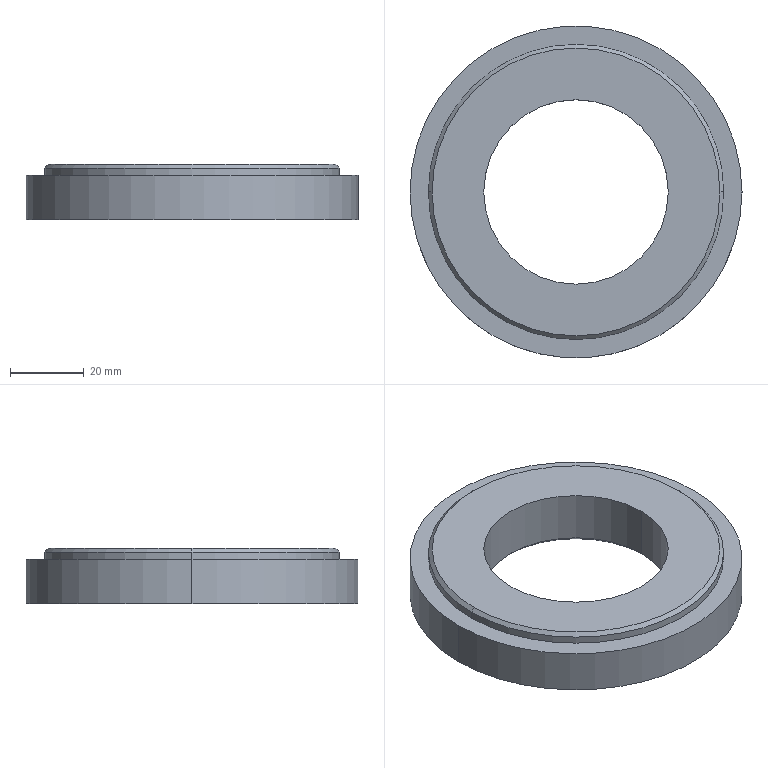Part | SolidWorks | features ICE 2, Chamfer 1, Extrusion 1 | 1 solid | 31 faces | box 90 x 90 x 15 mm | volume 60934 mm3 | cylinder 18 | plane 9 | cone 4 | commonest cylinder face diameters 4 x12 50 x2 80 x2 90 x2
STEP:
#1=CARTESIAN_POINT('',(39.,0.,15.));
#2=VERTEX_POINT('',#1);
#3=CARTESIAN_POINT('',(-39.,0.,15.));
#4=VERTEX_POINT('',#3);
#5=CARTESIAN_POINT('',(0.,0.,15.));
#6=DIRECTION('',(0.,0.,1.));
#7=DIRECTION('',(1.,0.,0.));
#8=AXIS2_PLACEMENT_3D('',#5,#6,#7);
#9=CIRCLE('',#8,39.);
#10=EDGE_CURVE('',#2,#4,#9,.T.);
#11=ORIENTED_EDGE('',*,*,#10,.F.);
#12=CARTESIAN_POINT('',(40.,0.,14.));
#13=VERTEX_POINT('',#12);
#14=CARTESIAN_POINT('',(39.,0.,15.));
#15=DIRECTION('',(0.7071,0.,-0.7071));
#16=VECTOR('',#15,1000.);
#17=LINE('',#14,#16);
#18=EDGE_CURVE('',#2,#13,#17,.T.);
#19=ORIENTED_EDGE('',*,*,#18,.T.);
#20=CARTESIAN_POINT('',(-40.,0.,14.));
#21=VERTEX_POINT('',#20);
#22=CARTESIAN_POINT('',(0.,0.,14.));
#23=DIRECTION('',(0.,0.,-1.));
#24=DIRECTION('',(1.,0.,0.));
#25=AXIS2_PLACEMENT_3D('',#22,#23,#24);
#26=CIRCLE('',#25,40.);
#27=EDGE_CURVE('',#21,#13,#26,.T.);
#28=ORIENTED_EDGE('',*,*,#27,.F.);
#29=CARTESIAN_POINT('',(-39.,0.,15.));
#30=DIRECTION('',(-0.7071,0.,-0.7071));
#31=VECTOR('',#30,1000.);
#32=LINE('',#29,#31);
#33=EDGE_CURVE('',#4,#21,#32,.T.);
#34=ORIENTED_EDGE('',*,*,#33,.F.);
#35=EDGE_LOOP('',(#11,#19,#28,#34));
#36=FACE_OUTER_BOUND('',#35,.T.);
#37=CARTESIAN_POINT('',(0.,0.,15.));
#38=DIRECTION('',(0.,0.,-1.));
#39=DIRECTION('',(-1.,0.,0.));
#40=AXIS2_PLACEMENT_3D('',#37,#38,#39);
#41=CONICAL_SURFACE('',#40,39.,0.7854);
#42=ADVANCED_FACE('',(#36),#41,.T.);
#43=CARTESIAN_POINT('',(25.,0.,1.));
#44=VERTEX_POINT('',#43);
#45=CARTESIAN_POINT('',(-25.,0.,1.));
#46=VERTEX_POINT('',#45);
#47=CARTESIAN_POINT('',(0.,0.,1.));
#48=DIRECTION('',(0.,0.,-1.));
#49=DIRECTION('',(1.,0.,0.));
#50=AXIS2_PLACEMENT_3D('',#47,#48,#49);
#51=CIRCLE('',#50,25.);
#52=EDGE_CURVE('',#44,#46,#51,.T.);
#53=ORIENTED_EDGE('',*,*,#52,.F.);
#54=CARTESIAN_POINT('',(26.,0.,0.));
#55=VERTEX_POINT('',#54);
#56=CARTESIAN_POINT('',(26.,0.,0.));
#57=DIRECTION('',(0.7071,0.,-0.7071));
#58=VECTOR('',#57,1000.);
#59=LINE('',#56,#58);
#60=EDGE_CURVE('',#44,#55,#59,.T.);
#61=ORIENTED_EDGE('',*,*,#60,.T.);
#62=CARTESIAN_POINT('',(-26.,0.,0.));
#63=VERTEX_POINT('',#62);
#64=CARTESIAN_POINT('',(0.,0.,0.));
#65=DIRECTION('',(0.,0.,1.));
#66=DIRECTION('',(1.,0.,0.));
#67=AXIS2_PLACEMENT_3D('',#64,#65,#66);
#68=CIRCLE('',#67,26.);
#69=EDGE_CURVE('',#63,#55,#68,.T.);
#70=ORIENTED_EDGE('',*,*,#69,.F.);
#71=CARTESIAN_POINT('',(-26.,0.,0.));
#72=DIRECTION('',(-0.7071,0.,-0.7071));
#73=VECTOR('',#72,1000.);
#74=LINE('',#71,#73);
#75=EDGE_CURVE('',#46,#63,#74,.T.);
#76=ORIENTED_EDGE('',*,*,#75,.F.);
#77=EDGE_LOOP('',(#53,#61,#70,#76));
#78=FACE_OUTER_BOUND('',#77,.T.);
#79=CARTESIAN_POINT('',(0.,0.,0.));
#80=DIRECTION('',(0.,0.,-1.));
#81=DIRECTION('',(-1.,0.,0.));
#82=AXIS2_PLACEMENT_3D('',#79,#80,#81);
#83=CONICAL_SURFACE('',#82,26.,0.7854);
#84=ADVANCED_FACE('',(#78),#83,.F.);
#85=CARTESIAN_POINT('',(33.61,18.25,11.));
#86=VERTEX_POINT('',#85);
#87=CARTESIAN_POINT('',(29.61,18.25,11.));
#88=VERTEX_POINT('',#87);
#89=CARTESIAN_POINT('',(31.61,18.25,11.));
#90=DIRECTION('',(0.,0.,-1.));
#91=DIRECTION('',(-1.,0.,0.));
#92=AXIS2_PLACEMENT_3D('',#89,#90,#91);
#93=CIRCLE('',#92,2.);
#94=EDGE_CURVE('',#86,#88,#93,.T.);
#95=ORIENTED_EDGE('',*,*,#94,.F.);
#96=CARTESIAN_POINT('',(33.61,18.25,0.));
#97=VERTEX_POINT('',#96);
#98=CARTESIAN_POINT('',(33.61,18.25,11.));
#99=DIRECTION('',(0.,0.,-1.));
#100=VECTOR('',#99,1000.);
#101=LINE('',#98,#100);
#102=EDGE_CURVE('',#86,#97,#101,.T.);
#103=ORIENTED_EDGE('',*,*,#102,.T.);
#104=CARTESIAN_POINT('',(29.61,18.25,0.));
#105=VERTEX_POINT('',#104);
#106=CARTESIAN_POINT('',(31.61,18.25,0.));
#107=DIRECTION('',(0.,0.,-1.));
#108=DIRECTION('',(-1.,0.,0.));
#109=AXIS2_PLACEMENT_3D('',#106,#107,#108);
#110=CIRCLE('',#109,2.);
#111=EDGE_CURVE('',#97,#105,#110,.T.);
#112=ORIENTED_EDGE('',*,*,#111,.T.);
#113=CARTESIAN_POINT('',(29.61,18.25,11.));
#114=DIRECTION('',(0.,0.,-1.));
#115=VECTOR('',#114,1000.);
#116=LINE('',#113,#115);
#117=EDGE_CURVE('',#88,#105,#116,.T.);
#118=ORIENTED_EDGE('',*,*,#117,.F.);
#119=EDGE_LOOP('',(#95,#103,#112,#118));
#120=FACE_OUTER_BOUND('',#119,.T.);
#121=CARTESIAN_POINT('',(31.61,18.25,11.));
#122=DIRECTION('',(0.,0.,-1.));
#123=DIRECTION('',(-1.,0.,0.));
#124=AXIS2_PLACEMENT_3D('',#121,#122,#123);
#125=CYLINDRICAL_SURFACE('',#124,2.);
#126=ADVANCED_FACE('',(#120),#125,.F.);
#127=CARTESIAN_POINT('',(33.61,-18.25,11.));
#128=VERTEX_POINT('',#127);
#129=CARTESIAN_POINT('',(29.61,-18.25,11.));
#130=VERTEX_POINT('',#129);
#131=CARTESIAN_POINT('',(31.61,-18.25,11.));
#132=DIRECTION('',(0.,0.,-1.));
#133=DIRECTION('',(-1.,0.,0.));
#134=AXIS2_PLACEMENT_3D('',#131,#132,#133);
#135=CIRCLE('',#134,2.);
#136=EDGE_CURVE('',#128,#130,#135,.T.);
#137=ORIENTED_EDGE('',*,*,#136,.F.);
#138=CARTESIAN_POINT('',(33.61,-18.25,0.));
#139=VERTEX_POINT('',#138);
#140=CARTESIAN_POINT('',(33.61,-18.25,11.));
#141=DIRECTION('',(0.,0.,-1.));
#142=VECTOR('',#141,1000.);
#143=LINE('',#140,#142);
#144=EDGE_CURVE('',#128,#139,#143,.T.);
#145=ORIENTED_EDGE('',*,*,#144,.T.);
#146=CARTESIAN_POINT('',(29.61,-18.25,0.));
#147=VERTEX_POINT('',#146);
#148=CARTESIAN_POINT('',(31.61,-18.25,0.));
#149=DIRECTION('',(0.,0.,-1.));
#150=DIRECTION('',(-1.,0.,0.));
#151=AXIS2_PLACEMENT_3D('',#148,#149,#150);
#152=CIRCLE('',#151,2.);
#153=EDGE_CURVE('',#139,#147,#152,.T.);
#154=ORIENTED_EDGE('',*,*,#153,.T.);
#155=CARTESIAN_POINT('',(29.61,-18.25,11.));
#156=DIRECTION('',(0.,0.,-1.));
#157=VECTOR('',#156,1000.);
#158=LINE('',#155,#157);
#159=EDGE_CURVE('',#130,#147,#158,.T.);
#160=ORIENTED_EDGE('',*,*,#159,.F.);
#161=EDGE_LOOP('',(#137,#145,#154,#160));
#162=FACE_OUTER_BOUND('',#161,.T.);
#163=CARTESIAN_POINT('',(31.61,-18.25,11.));
#164=DIRECTION('',(0.,0.,-1.));
#165=DIRECTION('',(-1.,0.,0.));
#166=AXIS2_PLACEMENT_3D('',#163,#164,#165);
#167=CYLINDRICAL_SURFACE('',#166,2.);
#168=ADVANCED_FACE('',(#162),#167,.F.);
#169=CARTESIAN_POINT('',(2.,-36.5,11.));
#170=VERTEX_POINT('',#169);
#171=CARTESIAN_POINT('',(-2.,-36.5,11.));
#172=VERTEX_POINT('',#171);
#173=CARTESIAN_POINT('',(0.,-36.5,11.));
#174=DIRECTION('',(0.,0.,-1.));
#175=DIRECTION('',(-1.,0.,0.));
#176=AXIS2_PLACEMENT_3D('',#173,#174,#175);
#177=CIRCLE('',#176,2.);
#178=EDGE_CURVE('',#170,#172,#177,.T.);
#179=ORIENTED_EDGE('',*,*,#178,.F.);
#180=CARTESIAN_POINT('',(2.,-36.5,0.));
#181=VERTEX_POINT('',#180);
#182=CARTESIAN_POINT('',(2.,-36.5,11.));
#183=DIRECTION('',(0.,0.,-1.));
#184=VECTOR('',#183,1000.);
#185=LINE('',#182,#184);
#186=EDGE_CURVE('',#170,#181,#185,.T.);
#187=ORIENTED_EDGE('',*,*,#186,.T.);
#188=CARTESIAN_POINT('',(-2.,-36.5,0.));
#189=VERTEX_POINT('',#188);
#190=CARTESIAN_POINT('',(0.,-36.5,0.));
#191=DIRECTION('',(0.,0.,-1.));
#192=DIRECTION('',(-1.,0.,0.));
#193=AXIS2_PLACEMENT_3D('',#190,#191,#192);
#194=CIRCLE('',#193,2.);
#195=EDGE_CURVE('',#181,#189,#194,.T.);
#196=ORIENTED_EDGE('',*,*,#195,.T.);
#197=CARTESIAN_POINT('',(-2.,-36.5,11.));
#198=DIRECTION('',(0.,0.,-1.));
#199=VECTOR('',#198,1000.);
#200=LINE('',#197,#199);
#201=EDGE_CURVE('',#172,#189,#200,.T.);
#202=ORIENTED_EDGE('',*,*,#201,.F.);
#203=EDGE_LOOP('',(#179,#187,#196,#202));
#204=FACE_OUTER_BOUND('',#203,.T.);
#205=CARTESIAN_POINT('',(0.,-36.5,11.));
#206=DIRECTION('',(0.,0.,-1.));
#207=DIRECTION('',(-1.,0.,0.));
#208=AXIS2_PLACEMENT_3D('',#205,#206,#207);
#209=CYLINDRICAL_SURFACE('',#208,2.);
#210=ADVANCED_FACE('',(#204),#209,.F.);
#211=CARTESIAN_POINT('',(-29.61,-18.25,11.));
#212=VERTEX_POINT('',#211);
#213=CARTESIAN_POINT('',(-33.61,-18.25,11.));
#214=VERTEX_POINT('',#213);
#215=CARTESIAN_POINT('',(-31.61,-18.25,11.));
#216=DIRECTION('',(0.,0.,-1.));
#217=DIRECTION('',(-1.,0.,0.));
#218=AXIS2_PLACEMENT_3D('',#215,#216,#217);
#219=CIRCLE('',#218,2.);
#220=EDGE_CURVE('',#212,#214,#219,.T.);
#221=ORIENTED_EDGE('',*,*,#220,.F.);
#222=CARTESIAN_POINT('',(-29.61,-18.25,0.));
#223=VERTEX_POINT('',#222);
#224=CARTESIAN_POINT('',(-29.61,-18.25,11.));
#225=DIRECTION('',(0.,0.,-1.));
#226=VECTOR('',#225,1000.);
#227=LINE('',#224,#226);
#228=EDGE_CURVE('',#212,#223,#227,.T.);
#229=ORIENTED_EDGE('',*,*,#228,.T.);
#230=CARTESIAN_POINT('',(-33.61,-18.25,0.));
#231=VERTEX_POINT('',#230);
#232=CARTESIAN_POINT('',(-31.61,-18.25,0.));
#233=DIRECTION('',(0.,0.,-1.));
#234=DIRECTION('',(-1.,0.,0.));
#235=AXIS2_PLACEMENT_3D('',#232,#233,#234);
#236=CIRCLE('',#235,2.);
#237=EDGE_CURVE('',#223,#231,#236,.T.);
#238=ORIENTED_EDGE('',*,*,#237,.T.);
#239=CARTESIAN_POINT('',(-33.61,-18.25,11.));
#240=DIRECTION('',(0.,0.,-1.));
#241=VECTOR('',#240,1000.);
#242=LINE('',#239,#241);
#243=EDGE_CURVE('',#214,#231,#242,.T.);
#244=ORIENTED_EDGE('',*,*,#243,.F.);
#245=EDGE_LOOP('',(#221,#229,#238,#244));
#246=FACE_OUTER_BOUND('',#245,.T.);
#247=CARTESIAN_POINT('',(-31.61,-18.25,11.));
#248=DIRECTION('',(0.,0.,-1.));
#249=DIRECTION('',(-1.,0.,0.));
#250=AXIS2_PLACEMENT_3D('',#247,#248,#249);
#251=CYLINDRICAL_SURFACE('',#250,2.);
#252=ADVANCED_FACE('',(#246),#251,.F.);
#253=CARTESIAN_POINT('',(-29.61,18.25,11.));
#254=VERTEX_POINT('',#253);
#255=CARTESIAN_POINT('',(-33.61,18.25,11.));
#256=VERTEX_POINT('',#255);
#257=CARTESIAN_POINT('',(-31.61,18.25,11.));
#258=DIRECTION('',(0.,0.,-1.));
#259=DIRECTION('',(-1.,0.,0.));
#260=AXIS2_PLACEMENT_3D('',#257,#258,#259);
#261=CIRCLE('',#260,2.);
#262=EDGE_CURVE('',#254,#256,#261,.T.);
#263=ORIENTED_EDGE('',*,*,#262,.F.);
#264=CARTESIAN_POINT('',(-29.61,18.25,0.));
#265=VERTEX_POINT('',#264);
#266=CARTESIAN_POINT('',(-29.61,18.25,11.));
#267=DIRECTION('',(0.,0.,-1.));
#268=VECTOR('',#267,1000.);
#269=LINE('',#266,#268);
#270=EDGE_CURVE('',#254,#265,#269,.T.);
#271=ORIENTED_EDGE('',*,*,#270,.T.);
#272=CARTESIAN_POINT('',(-33.61,18.25,0.));
#273=VERTEX_POINT('',#272);
#274=CARTESIAN_POINT('',(-31.61,18.25,0.));
#275=DIRECTION('',(0.,0.,-1.));
#276=DIRECTION('',(-1.,0.,0.));
#277=AXIS2_PLACEMENT_3D('',#274,#275,#276);
#278=CIRCLE('',#277,2.);
#279=EDGE_CURVE('',#265,#273,#278,.T.);
#280=ORIENTED_EDGE('',*,*,#279,.T.);
#281=CARTESIAN_POINT('',(-33.61,18.25,11.));
#282=DIRECTION('',(0.,0.,-1.));
#283=VECTOR('',#282,1000.);
#284=LINE('',#281,#283);
#285=EDGE_CURVE('',#256,#273,#284,.T.);
#286=ORIENTED_EDGE('',*,*,#285,.F.);
#287=EDGE_LOOP('',(#263,#271,#280,#286));
#288=FACE_OUTER_BOUND('',#287,.T.);
#289=CARTESIAN_POINT('',(-31.61,18.25,11.));
#290=DIRECTION('',(0.,0.,-1.));
#291=DIRECTION('',(-1.,0.,0.));
#292=AXIS2_PLACEMENT_3D('',#289,#290,#291);
#293=CYLINDRICAL_SURFACE('',#292,2.);
#294=ADVANCED_FACE('',(#288),#293,.F.);
#295=CARTESIAN_POINT('',(2.,36.5,11.));
#296=VERTEX_POINT('',#295);
#297=CARTESIAN_POINT('',(-2.,36.5,11.));
#298=VERTEX_POINT('',#297);
#299=CARTESIAN_POINT('',(0.,36.5,11.));
#300=DIRECTION('',(0.,0.,-1.));
#301=DIRECTION('',(-1.,0.,0.));
#302=AXIS2_PLACEMENT_3D('',#299,#300,#301);
#303=CIRCLE('',#302,2.);
#304=EDGE_CURVE('',#296,#298,#303,.T.);
#305=ORIENTED_EDGE('',*,*,#304,.F.);
#306=CARTESIAN_POINT('',(2.,36.5,0.));
#307=VERTEX_POINT('',#306);
#308=CARTESIAN_POINT('',(2.,36.5,11.));
#309=DIRECTION('',(0.,0.,-1.));
#310=VECTOR('',#309,1000.);
#311=LINE('',#308,#310);
#312=EDGE_CURVE('',#296,#307,#311,.T.);
#313=ORIENTED_EDGE('',*,*,#312,.T.);
#314=CARTESIAN_POINT('',(-2.,36.5,0.));
#315=VERTEX_POINT('',#314);
#316=CARTESIAN_POINT('',(0.,36.5,0.));
#317=DIRECTION('',(0.,0.,-1.));
#318=DIRECTION('',(-1.,0.,0.));
#319=AXIS2_PLACEMENT_3D('',#316,#317,#318);
#320=CIRCLE('',#319,2.);
#321=EDGE_CURVE('',#307,#315,#320,.T.);
#322=ORIENTED_EDGE('',*,*,#321,.T.);
#323=CARTESIAN_POINT('',(-2.,36.5,11.));
#324=DIRECTION('',(0.,0.,-1.));
#325=VECTOR('',#324,1000.);
#326=LINE('',#323,#325);
#327=EDGE_CURVE('',#298,#315,#326,.T.);
#328=ORIENTED_EDGE('',*,*,#327,.F.);
#329=EDGE_LOOP('',(#305,#313,#322,#328));
#330=FACE_OUTER_BOUND('',#329,.T.);
#331=CARTESIAN_POINT('',(0.,36.5,11.));
#332=DIRECTION('',(0.,0.,-1.));
#333=DIRECTION('',(-1.,0.,0.));
#334=AXIS2_PLACEMENT_3D('',#331,#332,#333);
#335=CYLINDRICAL_SURFACE('',#334,2.);
#336=ADVANCED_FACE('',(#330),#335,.F.);
#337=CARTESIAN_POINT('',(40.,0.,12.));
#338=VERTEX_POINT('',#337);
#339=CARTESIAN_POINT('',(-40.,0.,12.));
#340=VERTEX_POINT('',#339);
#341=CARTESIAN_POINT('',(0.,0.,12.));
#342=DIRECTION('',(0.,0.,1.));
#343=DIRECTION('',(1.,0.,0.));
#344=AXIS2_PLACEMENT_3D('',#341,#342,#343);
#345=CIRCLE('',#344,40.);
#346=EDGE_CURVE('',#338,#340,#345,.T.);
#347=ORIENTED_EDGE('',*,*,#346,.T.);
#348=CARTESIAN_POINT('',(-40.,0.,12.));
#349=DIRECTION('',(0.,0.,1.));
#350=VECTOR('',#349,1000.);
#351=LINE('',#348,#350);
#352=EDGE_CURVE('',#340,#21,#351,.T.);
#353=ORIENTED_EDGE('',*,*,#352,.T.);
#354=ORIENTED_EDGE('',*,*,#27,.T.);
#355=CARTESIAN_POINT('',(40.,0.,12.));
#356=DIRECTION('',(0.,0.,1.));
#357=VECTOR('',#356,1000.);
#358=LINE('',#355,#357);
#359=EDGE_CURVE('',#338,#13,#358,.T.);
#360=ORIENTED_EDGE('',*,*,#359,.F.);
#361=EDGE_LOOP('',(#347,#353,#354,#360));
#362=FACE_OUTER_BOUND('',#361,.T.);
#363=CARTESIAN_POINT('',(0.,0.,12.));
#364=DIRECTION('',(0.,0.,1.));
#365=DIRECTION('',(1.,0.,0.));
#366=AXIS2_PLACEMENT_3D('',#363,#364,#365);
#367=CYLINDRICAL_SURFACE('',#366,40.);
#368=ADVANCED_FACE('',(#362),#367,.T.);
#369=CARTESIAN_POINT('',(-25.,0.,15.));
#370=VERTEX_POINT('',#369);
#371=CARTESIAN_POINT('',(25.,0.,15.));
#372=VERTEX_POINT('',#371);
#373=CARTESIAN_POINT('',(0.,0.,15.));
#374=DIRECTION('',(0.,0.,1.));
#375=DIRECTION('',(1.,0.,0.));
#376=AXIS2_PLACEMENT_3D('',#373,#374,#375);
#377=CIRCLE('',#376,25.);
#378=EDGE_CURVE('',#370,#372,#377,.T.);
#379=ORIENTED_EDGE('',*,*,#378,.T.);
#380=CARTESIAN_POINT('',(25.,0.,15.));
#381=DIRECTION('',(0.,0.,-1.));
#382=VECTOR('',#381,1000.);
#383=LINE('',#380,#382);
#384=EDGE_CURVE('',#372,#44,#383,.T.);
#385=ORIENTED_EDGE('',*,*,#384,.T.);
#386=ORIENTED_EDGE('',*,*,#52,.T.);
#387=CARTESIAN_POINT('',(-25.,0.,15.));
#388=DIRECTION('',(0.,0.,-1.));
#389=VECTOR('',#388,1000.);
#390=LINE('',#387,#389);
#391=EDGE_CURVE('',#370,#46,#390,.T.);
#392=ORIENTED_EDGE('',*,*,#391,.F.);
#393=EDGE_LOOP('',(#379,#385,#386,#392));
#394=FACE_OUTER_BOUND('',#393,.T.);
#395=CARTESIAN_POINT('',(0.,0.,15.));
#396=DIRECTION('',(0.,0.,-1.));
#397=DIRECTION('',(-1.,0.,0.));
#398=AXIS2_PLACEMENT_3D('',#395,#396,#397);
#399=CYLINDRICAL_SURFACE('',#398,25.);
#400=ADVANCED_FACE('',(#394),#399,.F.);
#401=CARTESIAN_POINT('',(45.,0.,12.));
#402=VERTEX_POINT('',#401);
#403=CARTESIAN_POINT('',(-45.,0.,12.));
#404=VERTEX_POINT('',#403);
#405=CARTESIAN_POINT('',(0.,0.,12.));
#406=DIRECTION('',(0.,0.,1.));
#407=DIRECTION('',(1.,0.,0.));
#408=AXIS2_PLACEMENT_3D('',#405,#406,#407);
#409=CIRCLE('',#408,45.);
#410=EDGE_CURVE('',#402,#404,#409,.T.);
#411=ORIENTED_EDGE('',*,*,#410,.F.);
#412=CARTESIAN_POINT('',(45.,0.,0.));
#413=VERTEX_POINT('',#412);
#414=CARTESIAN_POINT('',(45.,0.,15.));
#415=DIRECTION('',(0.,0.,-1.));
#416=VECTOR('',#415,1000.);
#417=LINE('',#414,#416);
#418=EDGE_CURVE('',#402,#413,#417,.T.);
#419=ORIENTED_EDGE('',*,*,#418,.T.);
#420=CARTESIAN_POINT('',(-45.,0.,0.));
#421=VERTEX_POINT('',#420);
#422=CARTESIAN_POINT('',(0.,0.,0.));
#423=DIRECTION('',(0.,0.,1.));
#424=DIRECTION('',(1.,0.,0.));
#425=AXIS2_PLACEMENT_3D('',#422,#423,#424);
#426=CIRCLE('',#425,45.);
#427=EDGE_CURVE('',#413,#421,#426,.T.);
#428=ORIENTED_EDGE('',*,*,#427,.T.);
#429=CARTESIAN_POINT('',(-45.,0.,15.));
#430=DIRECTION('',(0.,0.,-1.));
#431=VECTOR('',#430,1000.);
#432=LINE('',#429,#431);
#433=EDGE_CURVE('',#404,#421,#432,.T.);
#434=ORIENTED_EDGE('',*,*,#433,.F.);
#435=EDGE_LOOP('',(#411,#419,#428,#434));
#436=FACE_OUTER_BOUND('',#435,.T.);
#437=CARTESIAN_POINT('',(0.,0.,15.));
#438=DIRECTION('',(0.,0.,-1.));
#439=DIRECTION('',(-1.,0.,0.));
#440=AXIS2_PLACEMENT_3D('',#437,#438,#439);
#441=CYLINDRICAL_SURFACE('',#440,45.);
#442=ADVANCED_FACE('',(#436),#441,.T.);
#443=CARTESIAN_POINT('',(0.,0.,15.));
#444=DIRECTION('',(0.,0.,1.));
#445=DIRECTION('',(1.,0.,0.));
#446=AXIS2_PLACEMENT_3D('',#443,#444,#445);
#447=CIRCLE('',#446,39.);
#448=EDGE_CURVE('',#4,#2,#447,.T.);
#449=ORIENTED_EDGE('',*,*,#448,.T.);
#450=ORIENTED_EDGE('',*,*,#10,.T.);
#451=EDGE_LOOP('',(#449,#450));
#452=FACE_OUTER_BOUND('',#451,.T.);
#453=ORIENTED_EDGE('',*,*,#378,.F.);
#454=CARTESIAN_POINT('',(0.,0.,15.));
#455=DIRECTION('',(0.,0.,1.));
#456=DIRECTION('',(1.,0.,0.));
#457=AXIS2_PLACEMENT_3D('',#454,#455,#456);
#458=CIRCLE('',#457,25.);
#459=EDGE_CURVE('',#372,#370,#458,.T.);
#460=ORIENTED_EDGE('',*,*,#459,.F.);
#461=EDGE_LOOP('',(#453,#460));
#462=FACE_BOUND('',#461,.T.);
#463=CARTESIAN_POINT('',(0.,0.,15.));
#464=DIRECTION('',(0.,0.,1.));
#465=DIRECTION('',(1.,0.,0.));
#466=AXIS2_PLACEMENT_3D('',#463,#464,#465);
#467=PLANE('',#466);
#468=ADVANCED_FACE('',(#452,#462),#467,.T.);
#469=ORIENTED_EDGE('',*,*,#418,.F.);
#470=CARTESIAN_POINT('',(0.,0.,12.));
#471=DIRECTION('',(0.,0.,1.));
#472=DIRECTION('',(1.,0.,0.));
#473=AXIS2_PLACEMENT_3D('',#470,#471,#472);
#474=CIRCLE('',#473,45.);
#475=EDGE_CURVE('',#404,#402,#474,.T.);
#476=ORIENTED_EDGE('',*,*,#475,.F.);
#477=ORIENTED_EDGE('',*,*,#433,.T.);
#478=CARTESIAN_POINT('',(0.,0.,0.));
#479=DIRECTION('',(0.,0.,1.));
#480=DIRECTION('',(1.,0.,0.));
#481=AXIS2_PLACEMENT_3D('',#478,#479,#480);
#482=CIRCLE('',#481,45.);
#483=EDGE_CURVE('',#421,#413,#482,.T.);
#484=ORIENTED_EDGE('',*,*,#483,.T.);
#485=EDGE_LOOP('',(#469,#476,#477,#484));
#486=FACE_OUTER_BOUND('',#485,.T.);
#487=CARTESIAN_POINT('',(0.,0.,15.));
#488=DIRECTION('',(0.,0.,-1.));
#489=DIRECTION('',(-1.,0.,0.));
#490=AXIS2_PLACEMENT_3D('',#487,#488,#489);
#491=CYLINDRICAL_SURFACE('',#490,45.);
#492=ADVANCED_FACE('',(#486),#491,.T.);
#493=ORIENTED_EDGE('',*,*,#69,.T.);
#494=CARTESIAN_POINT('',(0.,0.,0.));
#495=DIRECTION('',(0.,0.,1.));
#496=DIRECTION('',(1.,0.,0.));
#497=AXIS2_PLACEMENT_3D('',#494,#495,#496);
#498=CIRCLE('',#497,26.);
#499=EDGE_CURVE('',#55,#63,#498,.T.);
#500=ORIENTED_EDGE('',*,*,#499,.T.);
#501=EDGE_LOOP('',(#493,#500));
#502=FACE_BOUND('',#501,.T.);
#503=CARTESIAN_POINT('',(31.61,18.25,0.));
#504=DIRECTION('',(0.,0.,-1.));
#505=DIRECTION('',(-1.,0.,0.));
#506=AXIS2_PLACEMENT_3D('',#503,#504,#505);
#507=CIRCLE('',#506,2.);
#508=EDGE_CURVE('',#105,#97,#507,.T.);
#509=ORIENTED_EDGE('',*,*,#508,.F.);
#510=ORIENTED_EDGE('',*,*,#111,.F.);
#511=EDGE_LOOP('',(#509,#510));
#512=FACE_BOUND('',#511,.T.);
#513=CARTESIAN_POINT('',(31.61,-18.25,0.));
#514=DIRECTION('',(0.,0.,-1.));
#515=DIRECTION('',(-1.,0.,0.));
#516=AXIS2_PLACEMENT_3D('',#513,#514,#515);
#517=CIRCLE('',#516,2.);
#518=EDGE_CURVE('',#147,#139,#517,.T.);
#519=ORIENTED_EDGE('',*,*,#518,.F.);
#520=ORIENTED_EDGE('',*,*,#153,.F.);
#521=EDGE_LOOP('',(#519,#520));
#522=FACE_BOUND('',#521,.T.);
#523=CARTESIAN_POINT('',(0.,-36.5,0.));
#524=DIRECTION('',(0.,0.,-1.));
#525=DIRECTION('',(-1.,0.,0.));
#526=AXIS2_PLACEMENT_3D('',#523,#524,#525);
#527=CIRCLE('',#526,2.);
#528=EDGE_CURVE('',#189,#181,#527,.T.);
#529=ORIENTED_EDGE('',*,*,#528,.F.);
#530=ORIENTED_EDGE('',*,*,#195,.F.);
#531=EDGE_LOOP('',(#529,#530));
#532=FACE_BOUND('',#531,.T.);
#533=CARTESIAN_POINT('',(-31.61,-18.25,0.));
#534=DIRECTION('',(0.,0.,-1.));
#535=DIRECTION('',(-1.,0.,0.));
#536=AXIS2_PLACEMENT_3D('',#533,#534,#535);
#537=CIRCLE('',#536,2.);
#538=EDGE_CURVE('',#231,#223,#537,.T.);
#539=ORIENTED_EDGE('',*,*,#538,.F.);
#540=ORIENTED_EDGE('',*,*,#237,.F.);
#541=EDGE_LOOP('',(#539,#540));
#542=FACE_BOUND('',#541,.T.);
#543=CARTESIAN_POINT('',(-31.61,18.25,0.));
#544=DIRECTION('',(0.,0.,-1.));
#545=DIRECTION('',(-1.,0.,0.));
#546=AXIS2_PLACEMENT_3D('',#543,#544,#545);
#547=CIRCLE('',#546,2.);
#548=EDGE_CURVE('',#273,#265,#547,.T.);
#549=ORIENTED_EDGE('',*,*,#548,.F.);
#550=ORIENTED_EDGE('',*,*,#279,.F.);
#551=EDGE_LOOP('',(#549,#550));
#552=FACE_BOUND('',#551,.T.);
#553=CARTESIAN_POINT('',(0.,36.5,0.));
#554=DIRECTION('',(0.,0.,-1.));
#555=DIRECTION('',(-1.,0.,0.));
#556=AXIS2_PLACEMENT_3D('',#553,#554,#555);
#557=CIRCLE('',#556,2.);
#558=EDGE_CURVE('',#315,#307,#557,.T.);
#559=ORIENTED_EDGE('',*,*,#558,.F.);
#560=ORIENTED_EDGE('',*,*,#321,.F.);
#561=EDGE_LOOP('',(#559,#560));
#562=FACE_BOUND('',#561,.T.);
#563=ORIENTED_EDGE('',*,*,#483,.F.);
#564=ORIENTED_EDGE('',*,*,#427,.F.);
#565=EDGE_LOOP('',(#563,#564));
#566=FACE_OUTER_BOUND('',#565,.T.);
#567=CARTESIAN_POINT('',(0.,0.,0.));
#568=DIRECTION('',(0.,0.,1.));
#569=DIRECTION('',(1.,0.,0.));
#570=AXIS2_PLACEMENT_3D('',#567,#568,#569);
#571=PLANE('',#570);
#572=ADVANCED_FACE('',(#502,#512,#522,#532,#542,#552,#562,#566),#571,.F.);
#573=ORIENTED_EDGE('',*,*,#384,.F.);
#574=ORIENTED_EDGE('',*,*,#459,.T.);
#575=ORIENTED_EDGE('',*,*,#391,.T.);
#576=CARTESIAN_POINT('',(0.,0.,1.));
#577=DIRECTION('',(0.,0.,-1.));
#578=DIRECTION('',(1.,0.,0.));
#579=AXIS2_PLACEMENT_3D('',#576,#577,#578);
#580=CIRCLE('',#579,25.);
#581=EDGE_CURVE('',#46,#44,#580,.T.);
#582=ORIENTED_EDGE('',*,*,#581,.T.);
#583=EDGE_LOOP('',(#573,#574,#575,#582));
#584=FACE_OUTER_BOUND('',#583,.T.);
#585=CARTESIAN_POINT('',(0.,0.,15.));
#586=DIRECTION('',(0.,0.,-1.));
#587=DIRECTION('',(-1.,0.,0.));
#588=AXIS2_PLACEMENT_3D('',#585,#586,#587);
#589=CYLINDRICAL_SURFACE('',#588,25.);
#590=ADVANCED_FACE('',(#584),#589,.F.);
#591=ORIENTED_EDGE('',*,*,#346,.F.);
#592=CARTESIAN_POINT('',(0.,0.,12.));
#593=DIRECTION('',(0.,0.,1.));
#594=DIRECTION('',(1.,0.,0.));
#595=AXIS2_PLACEMENT_3D('',#592,#593,#594);
#596=CIRCLE('',#595,40.);
#597=EDGE_CURVE('',#340,#338,#596,.T.);
#598=ORIENTED_EDGE('',*,*,#597,.F.);
#599=EDGE_LOOP('',(#591,#598));
#600=FACE_BOUND('',#599,.T.);
#601=ORIENTED_EDGE('',*,*,#475,.T.);
#602=ORIENTED_EDGE('',*,*,#410,.T.);
#603=EDGE_LOOP('',(#601,#602));
#604=FACE_OUTER_BOUND('',#603,.T.);
#605=CARTESIAN_POINT('',(0.,0.,12.));
#606=DIRECTION('',(0.,0.,1.));
#607=DIRECTION('',(1.,0.,0.));
#608=AXIS2_PLACEMENT_3D('',#605,#606,#607);
#609=PLANE('',#608);
#610=ADVANCED_FACE('',(#600,#604),#609,.T.);
#611=ORIENTED_EDGE('',*,*,#352,.F.);
#612=ORIENTED_EDGE('',*,*,#597,.T.);
#613=ORIENTED_EDGE('',*,*,#359,.T.);
#614=CARTESIAN_POINT('',(0.,0.,14.));
#615=DIRECTION('',(0.,0.,-1.));
#616=DIRECTION('',(1.,0.,0.));
#617=AXIS2_PLACEMENT_3D('',#614,#615,#616);
#618=CIRCLE('',#617,40.);
#619=EDGE_CURVE('',#13,#21,#618,.T.);
#620=ORIENTED_EDGE('',*,*,#619,.T.);
#621=EDGE_LOOP('',(#611,#612,#613,#620));
#622=FACE_OUTER_BOUND('',#621,.T.);
#623=CARTESIAN_POINT('',(0.,0.,12.));
#624=DIRECTION('',(0.,0.,1.));
#625=DIRECTION('',(1.,0.,0.));
#626=AXIS2_PLACEMENT_3D('',#623,#624,#625);
#627=CYLINDRICAL_SURFACE('',#626,40.);
#628=ADVANCED_FACE('',(#622),#627,.T.);
#629=ORIENTED_EDGE('',*,*,#312,.F.);
#630=CARTESIAN_POINT('',(0.,36.5,11.));
#631=DIRECTION('',(0.,0.,-1.));
#632=DIRECTION('',(-1.,0.,0.));
#633=AXIS2_PLACEMENT_3D('',#630,#631,#632);
#634=CIRCLE('',#633,2.);
#635=EDGE_CURVE('',#298,#296,#634,.T.);
#636=ORIENTED_EDGE('',*,*,#635,.F.);
#637=ORIENTED_EDGE('',*,*,#327,.T.);
#638=ORIENTED_EDGE('',*,*,#558,.T.);
#639=EDGE_LOOP('',(#629,#636,#637,#638));
#640=FACE_OUTER_BOUND('',#639,.T.);
#641=CARTESIAN_POINT('',(0.,36.5,11.));
#642=DIRECTION('',(0.,0.,-1.));
#643=DIRECTION('',(-1.,0.,0.));
#644=AXIS2_PLACEMENT_3D('',#641,#642,#643);
#645=CYLINDRICAL_SURFACE('',#644,2.);
#646=ADVANCED_FACE('',(#640),#645,.F.);
#647=ORIENTED_EDGE('',*,*,#635,.T.);
#648=ORIENTED_EDGE('',*,*,#304,.T.);
#649=EDGE_LOOP('',(#647,#648));
#650=FACE_OUTER_BOUND('',#649,.T.);
#651=CARTESIAN_POINT('',(0.,36.5,11.));
#652=DIRECTION('',(0.,0.,-1.));
#653=DIRECTION('',(-1.,0.,0.));
#654=AXIS2_PLACEMENT_3D('',#651,#652,#653);
#655=PLANE('',#654);
#656=ADVANCED_FACE('',(#650),#655,.T.);
#657=ORIENTED_EDGE('',*,*,#270,.F.);
#658=CARTESIAN_POINT('',(-31.61,18.25,11.));
#659=DIRECTION('',(0.,0.,-1.));
#660=DIRECTION('',(-1.,0.,0.));
#661=AXIS2_PLACEMENT_3D('',#658,#659,#660);
#662=CIRCLE('',#661,2.);
#663=EDGE_CURVE('',#256,#254,#662,.T.);
#664=ORIENTED_EDGE('',*,*,#663,.F.);
#665=ORIENTED_EDGE('',*,*,#285,.T.);
#666=ORIENTED_EDGE('',*,*,#548,.T.);
#667=EDGE_LOOP('',(#657,#664,#665,#666));
#668=FACE_OUTER_BOUND('',#667,.T.);
#669=CARTESIAN_POINT('',(-31.61,18.25,11.));
#670=DIRECTION('',(0.,0.,-1.));
#671=DIRECTION('',(-1.,0.,0.));
#672=AXIS2_PLACEMENT_3D('',#669,#670,#671);
#673=CYLINDRICAL_SURFACE('',#672,2.);
#674=ADVANCED_FACE('',(#668),#673,.F.);
#675=ORIENTED_EDGE('',*,*,#663,.T.);
#676=ORIENTED_EDGE('',*,*,#262,.T.);
#677=EDGE_LOOP('',(#675,#676));
#678=FACE_OUTER_BOUND('',#677,.T.);
#679=CARTESIAN_POINT('',(-31.61,18.25,11.));
#680=DIRECTION('',(0.,0.,-1.));
#681=DIRECTION('',(-1.,0.,0.));
#682=AXIS2_PLACEMENT_3D('',#679,#680,#681);
#683=PLANE('',#682);
#684=ADVANCED_FACE('',(#678),#683,.T.);
#685=ORIENTED_EDGE('',*,*,#228,.F.);
#686=CARTESIAN_POINT('',(-31.61,-18.25,11.));
#687=DIRECTION('',(0.,0.,-1.));
#688=DIRECTION('',(-1.,0.,0.));
#689=AXIS2_PLACEMENT_3D('',#686,#687,#688);
#690=CIRCLE('',#689,2.);
#691=EDGE_CURVE('',#214,#212,#690,.T.);
#692=ORIENTED_EDGE('',*,*,#691,.F.);
#693=ORIENTED_EDGE('',*,*,#243,.T.);
#694=ORIENTED_EDGE('',*,*,#538,.T.);
#695=EDGE_LOOP('',(#685,#692,#693,#694));
#696=FACE_OUTER_BOUND('',#695,.T.);
#697=CARTESIAN_POINT('',(-31.61,-18.25,11.));
#698=DIRECTION('',(0.,0.,-1.));
#699=DIRECTION('',(-1.,0.,0.));
#700=AXIS2_PLACEMENT_3D('',#697,#698,#699);
#701=CYLINDRICAL_SURFACE('',#700,2.);
#702=ADVANCED_FACE('',(#696),#701,.F.);
#703=ORIENTED_EDGE('',*,*,#691,.T.);
#704=ORIENTED_EDGE('',*,*,#220,.T.);
#705=EDGE_LOOP('',(#703,#704));
#706=FACE_OUTER_BOUND('',#705,.T.);
#707=CARTESIAN_POINT('',(-31.61,-18.25,11.));
#708=DIRECTION('',(0.,0.,-1.));
#709=DIRECTION('',(-1.,0.,0.));
#710=AXIS2_PLACEMENT_3D('',#707,#708,#709);
#711=PLANE('',#710);
#712=ADVANCED_FACE('',(#706),#711,.T.);
#713=ORIENTED_EDGE('',*,*,#186,.F.);
#714=CARTESIAN_POINT('',(0.,-36.5,11.));
#715=DIRECTION('',(0.,0.,-1.));
#716=DIRECTION('',(-1.,0.,0.));
#717=AXIS2_PLACEMENT_3D('',#714,#715,#716);
#718=CIRCLE('',#717,2.);
#719=EDGE_CURVE('',#172,#170,#718,.T.);
#720=ORIENTED_EDGE('',*,*,#719,.F.);
#721=ORIENTED_EDGE('',*,*,#201,.T.);
#722=ORIENTED_EDGE('',*,*,#528,.T.);
#723=EDGE_LOOP('',(#713,#720,#721,#722));
#724=FACE_OUTER_BOUND('',#723,.T.);
#725=CARTESIAN_POINT('',(0.,-36.5,11.));
#726=DIRECTION('',(0.,0.,-1.));
#727=DIRECTION('',(-1.,0.,0.));
#728=AXIS2_PLACEMENT_3D('',#725,#726,#727);
#729=CYLINDRICAL_SURFACE('',#728,2.);
#730=ADVANCED_FACE('',(#724),#729,.F.);
#731=ORIENTED_EDGE('',*,*,#719,.T.);
#732=ORIENTED_EDGE('',*,*,#178,.T.);
#733=EDGE_LOOP('',(#731,#732));
#734=FACE_OUTER_BOUND('',#733,.T.);
#735=CARTESIAN_POINT('',(0.,-36.5,11.));
#736=DIRECTION('',(0.,0.,-1.));
#737=DIRECTION('',(-1.,0.,0.));
#738=AXIS2_PLACEMENT_3D('',#735,#736,#737);
#739=PLANE('',#738);
#740=ADVANCED_FACE('',(#734),#739,.T.);
#741=ORIENTED_EDGE('',*,*,#144,.F.);
#742=CARTESIAN_POINT('',(31.61,-18.25,11.));
#743=DIRECTION('',(0.,0.,-1.));
#744=DIRECTION('',(-1.,0.,0.));
#745=AXIS2_PLACEMENT_3D('',#742,#743,#744);
#746=CIRCLE('',#745,2.);
#747=EDGE_CURVE('',#130,#128,#746,.T.);
#748=ORIENTED_EDGE('',*,*,#747,.F.);
#749=ORIENTED_EDGE('',*,*,#159,.T.);
#750=ORIENTED_EDGE('',*,*,#518,.T.);
#751=EDGE_LOOP('',(#741,#748,#749,#750));
#752=FACE_OUTER_BOUND('',#751,.T.);
#753=CARTESIAN_POINT('',(31.61,-18.25,11.));
#754=DIRECTION('',(0.,0.,-1.));
#755=DIRECTION('',(-1.,0.,0.));
#756=AXIS2_PLACEMENT_3D('',#753,#754,#755);
#757=CYLINDRICAL_SURFACE('',#756,2.);
#758=ADVANCED_FACE('',(#752),#757,.F.);
#759=ORIENTED_EDGE('',*,*,#747,.T.);
#760=ORIENTED_EDGE('',*,*,#136,.T.);
#761=EDGE_LOOP('',(#759,#760));
#762=FACE_OUTER_BOUND('',#761,.T.);
#763=CARTESIAN_POINT('',(31.61,-18.25,11.));
#764=DIRECTION('',(0.,0.,-1.));
#765=DIRECTION('',(-1.,0.,0.));
#766=AXIS2_PLACEMENT_3D('',#763,#764,#765);
#767=PLANE('',#766);
#768=ADVANCED_FACE('',(#762),#767,.T.);
#769=ORIENTED_EDGE('',*,*,#102,.F.);
#770=CARTESIAN_POINT('',(31.61,18.25,11.));
#771=DIRECTION('',(0.,0.,-1.));
#772=DIRECTION('',(-1.,0.,0.));
#773=AXIS2_PLACEMENT_3D('',#770,#771,#772);
#774=CIRCLE('',#773,2.);
#775=EDGE_CURVE('',#88,#86,#774,.T.);
#776=ORIENTED_EDGE('',*,*,#775,.F.);
#777=ORIENTED_EDGE('',*,*,#117,.T.);
#778=ORIENTED_EDGE('',*,*,#508,.T.);
#779=EDGE_LOOP('',(#769,#776,#777,#778));
#780=FACE_OUTER_BOUND('',#779,.T.);
#781=CARTESIAN_POINT('',(31.61,18.25,11.));
#782=DIRECTION('',(0.,0.,-1.));
#783=DIRECTION('',(-1.,0.,0.));
#784=AXIS2_PLACEMENT_3D('',#781,#782,#783);
#785=CYLINDRICAL_SURFACE('',#784,2.);
#786=ADVANCED_FACE('',(#780),#785,.F.);
#787=ORIENTED_EDGE('',*,*,#775,.T.);
#788=ORIENTED_EDGE('',*,*,#94,.T.);
#789=EDGE_LOOP('',(#787,#788));
#790=FACE_OUTER_BOUND('',#789,.T.);
#791=CARTESIAN_POINT('',(31.61,18.25,11.));
#792=DIRECTION('',(0.,0.,-1.));
#793=DIRECTION('',(-1.,0.,0.));
#794=AXIS2_PLACEMENT_3D('',#791,#792,#793);
#795=PLANE('',#794);
#796=ADVANCED_FACE('',(#790),#795,.T.);
#797=ORIENTED_EDGE('',*,*,#60,.F.);
#798=ORIENTED_EDGE('',*,*,#581,.F.);
#799=ORIENTED_EDGE('',*,*,#75,.T.);
#800=ORIENTED_EDGE('',*,*,#499,.F.);
#801=EDGE_LOOP('',(#797,#798,#799,#800));
#802=FACE_OUTER_BOUND('',#801,.T.);
#803=CARTESIAN_POINT('',(0.,0.,0.));
#804=DIRECTION('',(0.,0.,-1.));
#805=DIRECTION('',(-1.,0.,0.));
#806=AXIS2_PLACEMENT_3D('',#803,#804,#805);
#807=CONICAL_SURFACE('',#806,26.,0.7854);
#808=ADVANCED_FACE('',(#802),#807,.F.);
#809=ORIENTED_EDGE('',*,*,#18,.F.);
#810=ORIENTED_EDGE('',*,*,#448,.F.);
#811=ORIENTED_EDGE('',*,*,#33,.T.);
#812=ORIENTED_EDGE('',*,*,#619,.F.);
#813=EDGE_LOOP('',(#809,#810,#811,#812));
#814=FACE_OUTER_BOUND('',#813,.T.);
#815=CARTESIAN_POINT('',(0.,0.,15.));
#816=DIRECTION('',(0.,0.,-1.));
#817=DIRECTION('',(-1.,0.,0.));
#818=AXIS2_PLACEMENT_3D('',#815,#816,#817);
#819=CONICAL_SURFACE('',#818,39.,0.7854);
#820=ADVANCED_FACE('',(#814),#819,.T.);
#821=CLOSED_SHELL('',(#42,#84,#126,#168,#210,#252,#294,#336,#368,#400,#442,#468,#492,#572,#590,#610,#628,#646,#656,#674,#684,#702,#712,#730,#740,#758,#768,#786,#796,#808,#820));
#822=MANIFOLD_SOLID_BREP('',#821);
#823=CARTESIAN_POINT('',(0.,0.,0.));
#824=DIRECTION('',(0.,0.,1.));
#825=DIRECTION('',(1.,0.,0.));
#826=AXIS2_PLACEMENT_3D('',#823,#824,#825);
#827=(LENGTH_UNIT()NAMED_UNIT(*)SI_UNIT(.MILLI.,.METRE.));
#828=UNCERTAINTY_MEASURE_WITH_UNIT(LENGTH_MEASURE(0.00001),#827,'','');
#829=(NAMED_UNIT(*)PLANE_ANGLE_UNIT()SI_UNIT($,.RADIAN.));
#830=(NAMED_UNIT(*)SI_UNIT($,.STERADIAN.)SOLID_ANGLE_UNIT());
#831=(GEOMETRIC_REPRESENTATION_CONTEXT(3)GLOBAL_UNCERTAINTY_ASSIGNED_CONTEXT((#828))GLOBAL_UNIT_ASSIGNED_CONTEXT((#827,#829,#830))REPRESENTATION_CONTEXT('',''));
#832=ADVANCED_BREP_SHAPE_REPRESENTATION('',(#822,#826),#831);